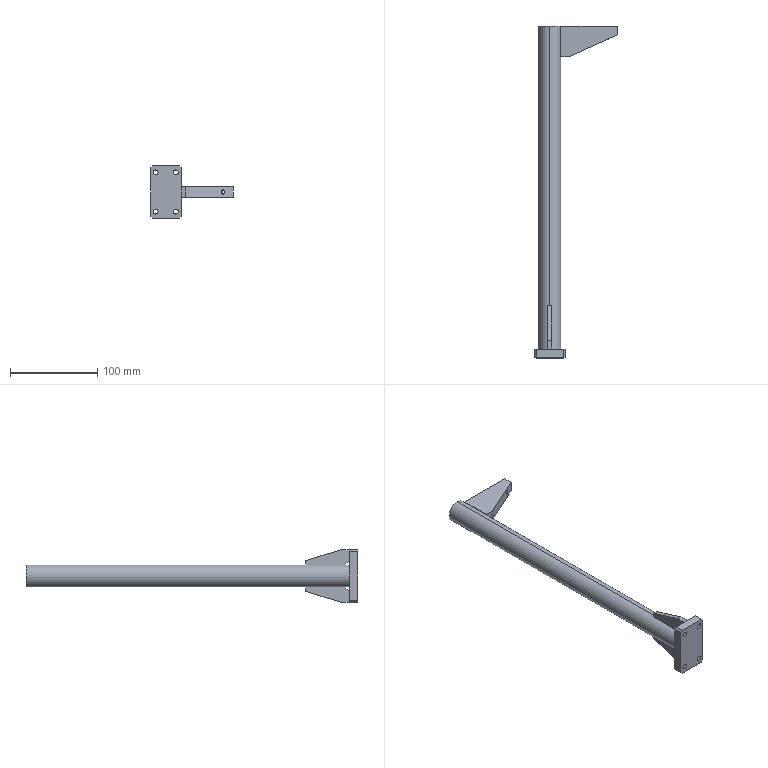Part | SolidWorks | features HoleWzd 3, ICE 3, Chamfer 1, Extrusion 1 | 5 solids | 58 faces | box 95 x 380 x 60 mm | volume 225421 mm3 | plane 35 | cylinder 16 | cone 7 | commonest cylinder face diameters 5.5 x8 5 x4 6.8 x2 25 x2